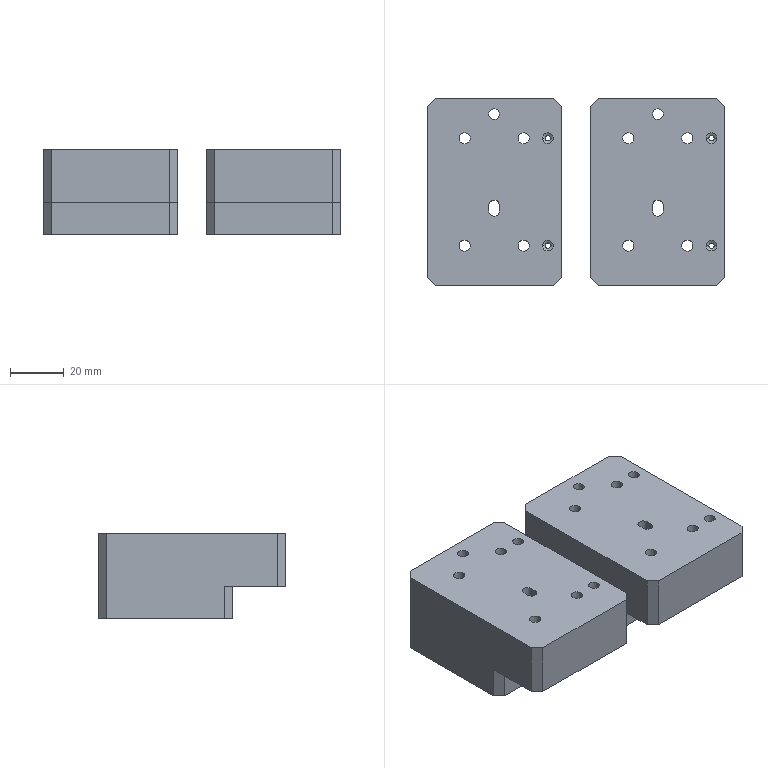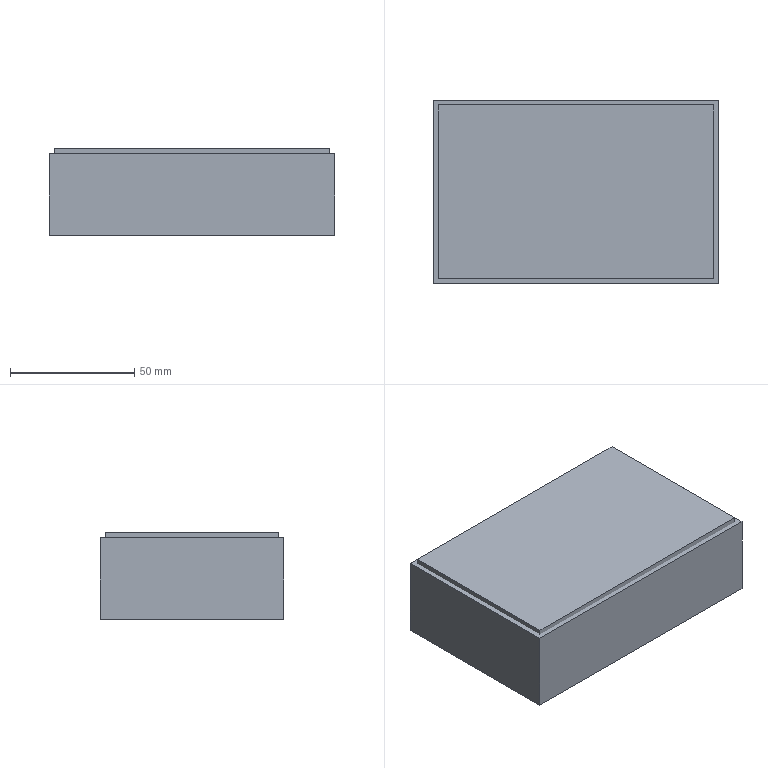CAM job | NX | 3-axis milling, drilling | part box 111 x 70 x 32 mm | stock box 115 x 74 x 35 mm
Tools:
number,name,description,diameter,corner_radius,flute_length,length,flutes
19,D80,Milling Tool-5 Parameters,80.0,0.0,50.0,75.0,2
15,D10,Milling Tool-5 Parameters,10.0,0.0,50.0,75.0,2
14,D10JING,Milling Tool-5 Parameters,10.0,0.0,50.0,75.0,2
1,D6A45,Milling Tool-5 Parameters,6.0,0.0,50.0,75.0,2
4,4.2ZT,Drilling Tool,4.2,0.0,35.0,50.0,2
18,3.4ZT,Drilling Tool,3.4,0.0,35.0,50.0,2
17,2.0ZT,Drilling Tool,2.0,0.0,35.0,50.0,2
3,D3,Milling Tool-5 Parameters,3.0,1.0,30.0,30.0,4
Operations:
program,operation,operation_type,tool,method,geometry_group,spindle_rpm,surface_speed,feed_per_tooth,feed_cut,feed_plunge,cut_length_mm,path_length_mm,cut_time_min,machine_time_min
1,FLOOR_WALL,VolumeBased25DMillingOperation,D80,METHOD,A,6500.0,1633.0,0.1154,1500.0,100.0,207.0,261.0,0.138,0.1434
1,ZLEVEL_PROFILE,ZLevelMilling,D10,METHOD,A,9500.0,298.0,0.1579,3000.0,1000.0,17588.833,17929.608,5.927,5.961
1,ZLEVEL_PROFILE_1,ZLevelMilling,D10JING,METHOD,A,9500.0,298.0,0.0789,1500.0,1000.0,1347.428,2034.851,0.9023,0.9711
1,DRILLING,Operation,D6A45,METHOD,A,9500.0,179.0,0.0132,250.0,0.0,76.8,518.337,0.3072,0.3514
1,DRILLING_COPY_COPY,Operation,4.2ZT,METHOD,A,2000.0,21.0,0.0375,150.0,0.0,254.095,796.346,1.694,1.748
1,DRILLING_COPY_COPY_1,Operation,3.4ZT,METHOD,A,2000.0,21.0,0.0375,150.0,0.0,194.893,718.621,1.299,1.352
1,DRILLING_COPY_COPY_1_COPY,Operation,2.0ZT,METHOD,A,2000.0,12.0,0.02,80.0,0.0,124.403,471.038,1.555,1.59
1,HOLE_MILLING,CylinderMilling,D3,METHOD,A,9500.0,89.0,0.0329,1250.0,100.0,393.262,800.263,0.3146,0.3553
1,PLANAR_MILL_COPY,PlanarMilling,D6A45,METHOD,A,9500.0,179.0,0.0658,1250.0,100.0,636.537,1740.124,0.5092,0.6196
1,刀补3,CylinderMilling,D3,METHOD,A,9500.0,89.0,0.0329,1250.0,100.0,68.854,475.854,0.0551,0.0958
2,FLOOR_WALL_COPY,VolumeBased25DMillingOperation,D80,METHOD,B,6500.0,1633.0,0.1154,1500.0,100.0,609.0,1159.001,0.406,0.461
2,FLOOR_WALL_1,VolumeBased25DMillingOperation,D10,METHOD,B,9500.0,298.0,0.1842,3500.0,1000.0,9241.979,9683.461,2.704,2.748
2,FLOOR_WALL_1_COPY,VolumeBased25DMillingOperation,D10JING,METHOD,B,9500.0,298.0,0.0789,1500.0,1000.0,669.303,1096.804,0.4528,0.4955
2,PLANAR_MILL_COPY_COPY,PlanarMilling,D6A45,METHOD,B,9500.0,179.0,0.0658,1250.0,100.0,543.55,1808.452,0.4348,0.5613
2,PLANAR_MILL_COPY_COPY_COPY,PlanarMilling,D6A45,METHOD,B,9500.0,179.0,0.0658,1250.0,100.0,266.841,1145.128,0.2135,0.3013